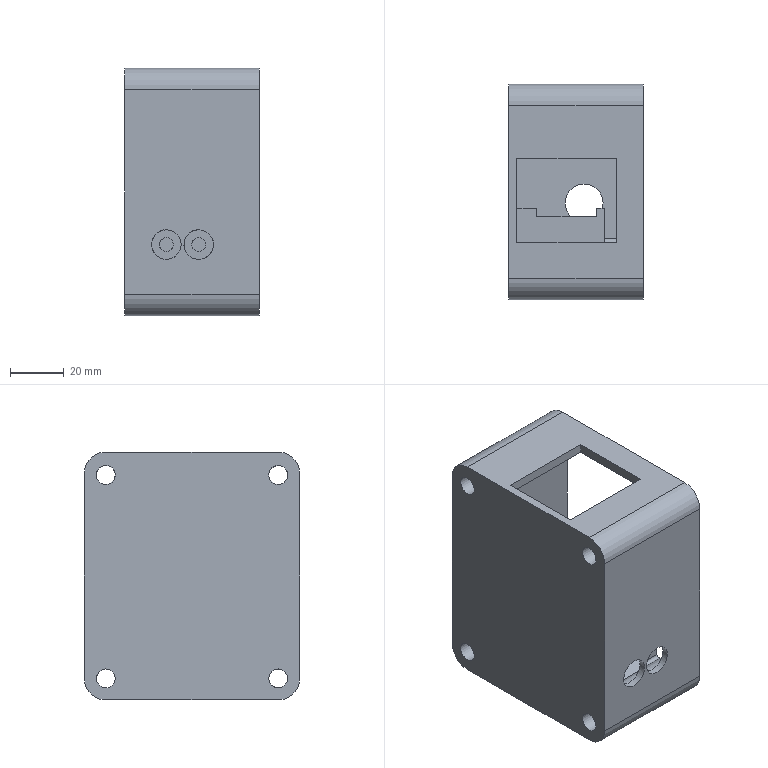NC program | NX | posted by the shop | part box 50 x 80 x 92 mm
Lines 26784 to 27158 of 30419:
(T=11 N=D6-18-D6-50-3T-rough D=6.00 R=0.00 FL=18.00 L=50.00)
(XY-STOCK=0.00)
T11 M6
T15
G0 G90 G54 X-1.75 Y-32.5 S4000 M3
G43 H11 Z30.
M8
Z-5.5
G1 Z-7.5 F800.
G3 X.25 Y-34.5 I2. J0.0
G1 X27.802
G2 X32.762 Y-22.9 I10.198 J2.5
X34.258 Y-22.5 I1.497 J-2.6
G1 X40.
Y22.5
X34.258
G2 X32.762 Y22.9 I0.0 J3.
X27.802 Y34.5 I5.238 J9.1
G1 X-27.302
G2 X-32.262 Y22.9 I-10.198 J-2.5
X-33.758 Y22.5 I-1.497 J2.6
G1 X-41.
Y-22.5
X-33.758
G2 X-32.262 Y-22.9 I0.0 J-3.
X-27.302 Y-34.5 I-5.238 J-9.1
G1 X.25
G3 X2.25 Y-32.5 I0.0 J2.
G1 Z-5.5
G0 Z30.
G0 X31.922 Y14. S4000 M3
M8
Z-5.5
G1 Z-7.5 F800.
Y18.
G3 X29.922 Y20. I-2. J0.0
G1 X-29.422
G3 X-31.422 Y18. I0.0 J-2.
G1 Y14.
Z-5.5
G0 Z30.
X31.922
Z-5.5
G1 Z-7.5
Y21.
G3 X29.922 Y23. I-2. J0.0
G1 X-29.422
G3 X-31.422 Y21. I0.0 J-2.
G1 Y14.
Z-5.5
G0 Z30.
Y-14.
Z-5.5
G1 Z-7.5
Y-18.
G3 X-29.422 Y-20. I2. J0.0
G1 X31.979
G3 X33.979 Y-18. I0.0 J2.
G1 Y-14.
Z-5.5
G0 Z30.
X-31.422
Z-5.5
G1 Z-7.5
Y-21.
G3 X-29.422 Y-23. I2. J0.0
G1 X31.979
G3 X33.979 Y-21. I0.0 J2.
G1 Y-14.
Z-5.5
G0 Z30.
G0 X-.75 Y-33.5 S4000 M3
M8
Z-15.
G1 Z-17. F800.
G3 X.25 Y-34.5 I1. J0.0
G1 X27.802
G2 X28.014 Y-28.756 I10.198 J2.5
G1 X27.257 Y-28.
X-27.792
G2 X-27.302 Y-34.5 I-9.708 J-4.
G1 X.25
G3 X1.25 Y-33.5 I0.0 J1.
G1 X-.75
G3 X.25 Y-34.5 I1. J0.0
G1 X27.802
G2 X28.014 Y-28.756 I10.198 J2.5
G1 X27.257 Y-28.
X-27.792
G2 X-27.302 Y-34.5 I-9.708 J-4.
G1 X.25
G3 X1.25 Y-33.5 I0.0 J1.
G1 Z-15.
G0 Z30.
Y33.5
Z-15.
G1 Z-17.
G3 X.25 Y34.5 I-1. J0.0
G1 X-27.302
G2 X-27.792 Y28. I-10.198 J-2.5
G1 X28.292
G2 X27.802 Y34.5 I9.708 J4.
G1 X.25
G3 X-.75 Y33.5 I0.0 J-1.
G1 X1.25
G3 X.25 Y34.5 I-1. J0.0
G1 X-27.302
G2 X-27.792 Y28. I-10.198 J-2.5
G1 X28.292
G2 X27.802 Y34.5 I9.708 J4.
G1 X.25
G3 X-.75 Y33.5 I0.0 J-1.
G1 Z-15.
G0 Z30.
G0 X3. Y-.402 S4000 M3
M8
Z-11.5
G1 Z-14.5 F800.
Y-6.
G3 X4.5 Y-7.5 I1.5 J0.0
G1 X30.5
Y-11.333
X4.5
Y-15.167
X30.5
X31.743 Y-19.
X4.696
Z-11.5
G0 Z30.
M9
M5
G91 G28 Z0.0
M1
N9
(T=15 N=D6-18-D6-50-3T-rough D=6.00 R=0.00 FL=18.00 L=50.00)
(XY-STOCK=0.00)
T15 M6
T8
G0 G90 G54 X-37.5 Y2. S4000 M3
G43 H15 Z30.
M8
Z-45.
G1 Z-47. F800.
G3 X-39.5 Y0.0 I0.0 J-2.
G1 Y-16.084
G2 X-35.304 Y-19. I-1. J-5.916
G1 X-5.696
G2 X4.104 Y-18.153 I5.196 J-3.
G1 X4.5 Y-17.757
Y-6.
G2 X7.5 Y-3. I3. J0.0
G1 X27.5
G2 X30.5 Y-6. I0.0 J-3.
G1 Y-17.757
X31.743 Y-19.
X34.304
G2 X38.5 Y-16.084 I5.196 J-3.
G1 Y16.084
G2 X34.304 Y19. I1. J5.916
G1 X4.696
G2 X-5.696 I-5.196 J3.
G1 X-35.304
G2 X-39.5 Y16.084 I-5.196 J3.
G1 Y0.0
G3 X-37.5 Y-2. I2. J0.0
G1 Y2.
G3 X-39.5 Y0.0 I0.0 J-2.
G1 Y-16.084
G2 X-35.304 Y-19. I-1. J-5.916
G1 X-5.696
G2 X4.104 Y-18.153 I5.196 J-3.
G1 X4.5 Y-17.757
Y-6.
G2 X7.5 Y-3. I3. J0.0
G1 X27.5
G2 X30.5 Y-6. I0.0 J-3.
G1 Y-17.757
X31.743 Y-19.
X34.304
G2 X38.5 Y-16.084 I5.196 J-3.
G1 Y16.084
G2 X34.304 Y19. I1. J5.916
G1 X4.696
G2 X-5.696 I-5.196 J3.
G1 X-35.304
G2 X-39.5 Y16.084 I-5.196 J3.
G1 Y0.0
G3 X-37.5 Y-2. I2. J0.0
G1 Y2.
G3 X-39.5 Y0.0 I0.0 J-2.
G1 Y-16.084
G2 X-35.304 Y-19. I-1. J-5.916
G1 X-5.696
G2 X4.104 Y-18.153 I5.196 J-3.
G1 X4.5 Y-17.757
Y-6.
G2 X7.5 Y-3. I3. J0.0
G1 X27.5
G2 X30.5 Y-6. I0.0 J-3.
G1 Y-17.757
X31.743 Y-19.
X34.304
G2 X38.5 Y-16.084 I5.196 J-3.
G1 Y16.084
G2 X34.304 Y19. I1. J5.916
G1 X4.696
G2 X-5.696 I-5.196 J3.
G1 X-35.304
G2 X-39.5 Y16.084 I-5.196 J3.
G1 Y0.0
G3 X-37.5 Y-2. I2. J0.0
G1 Y2.
G3 X-39.5 Y0.0 I0.0 J-2.
G1 Y-16.084
G2 X-35.304 Y-19. I-1. J-5.916
G1 X-5.696
G2 X4.104 Y-18.153 I5.196 J-3.
G1 X4.5 Y-17.757
Y-6.
G2 X7.5 Y-3. I3. J0.0
G1 X27.5
G2 X30.5 Y-6. I0.0 J-3.
G1 Y-17.757
X31.743 Y-19.
X34.304
G2 X38.5 Y-16.084 I5.196 J-3.
G1 Y16.084
G2 X34.304 Y19. I1. J5.916
G1 X4.696
G2 X-5.696 I-5.196 J3.
G1 X-35.304
G2 X-39.5 Y16.084 I-5.196 J3.
G1 Y0.0
G3 X-37.5 Y-2. I2. J0.0
G1 Y2.
G3 X-39.5 Y0.0 I0.0 J-2.
G1 Y-16.084
G2 X-35.304 Y-19. I-1. J-5.916
G1 X-5.696
G2 X4.104 Y-18.153 I5.196 J-3.
G1 X4.5 Y-17.757
Y-6.
G2 X7.5 Y-3. I3. J0.0
G1 X27.5
G2 X30.5 Y-6. I0.0 J-3.
G1 Y-17.757
X31.743 Y-19.
X34.304
G2 X38.5 Y-16.084 I5.196 J-3.
G1 Y16.084
G2 X34.304 Y19. I1. J5.916
G1 X4.696
G2 X-5.696 I-5.196 J3.
G1 X-35.304
G2 X-39.5 Y16.084 I-5.196 J3.
G1 Y0.0
G3 X-37.5 Y-2. I2. J0.0
G1 Z-45.
G0 Z30.
G0 X-.75 Y-33.5 S4000 M3
M8
Z-45.
G1 Z-47. F800.
G3 X.25 Y-34.5 I1. J0.0
G1 X27.802
G2 X28.014 Y-28.756 I10.198 J2.5
G1 X27.257 Y-28.
X-27.792
G2 X-27.302 Y-34.5 I-9.708 J-4.
G1 X.25
G3 X1.25 Y-33.5 I0.0 J1.
G1 X-.75
G3 X.25 Y-34.5 I1. J0.0
G1 X27.802
G2 X28.014 Y-28.756 I10.198 J2.5
G1 X27.257 Y-28.
X-27.792
G2 X-27.302 Y-34.5 I-9.708 J-4.
G1 X.25
G3 X1.25 Y-33.5 I0.0 J1.
G1 X-.75
G3 X.25 Y-34.5 I1. J0.0
G1 X27.802
G2 X28.014 Y-28.756 I10.198 J2.5
G1 X27.257 Y-28.
X-27.792
G2 X-27.302 Y-34.5 I-9.708 J-4.
G1 X.25
G3 X1.25 Y-33.5 I0.0 J1.
G1 X-.75
G3 X.25 Y-34.5 I1. J0.0
G1 X27.802
G2 X28.014 Y-28.756 I10.198 J2.5
G1 X27.257 Y-28.
X-27.792
G2 X-27.302 Y-34.5 I-9.708 J-4.
G1 X.25
G3 X1.25 Y-33.5 I0.0 J1.
G1 X-.75
G3 X.25 Y-34.5 I1. J0.0
G1 X27.802
G2 X28.014 Y-28.756 I10.198 J2.5
G1 X27.257 Y-28.
X-27.792
G2 X-27.302 Y-34.5 I-9.708 J-4.
G1 X.25
G3 X1.25 Y-33.5 I0.0 J1.
G1 X-.75
G3 X.25 Y-34.5 I1. J0.0
G1 X27.802
G2 X28.014 Y-28.756 I10.198 J2.5
G1 X27.257 Y-28.
X-27.792
G2 X-27.302 Y-34.5 I-9.708 J-4.
G1 X.25
G3 X1.25 Y-33.5 I0.0 J1.
G1 Z-45.
G0 Z30.
Y33.5
Z-45.
G1 Z-47.
G3 X.25 Y34.5 I-1. J0.0
G1 X-27.302
G2 X-27.792 Y28. I-10.198 J-2.5
G1 X28.292
G2 X27.802 Y34.5 I9.708 J4.
G1 X.25
G3 X-.75 Y33.5 I0.0 J-1.
G1 X1.25
G3 X.25 Y34.5 I-1. J0.0
G1 X-27.302
G2 X-27.792 Y28. I-10.198 J-2.5
G1 X28.292
G2 X27.802 Y34.5 I9.708 J4.
G1 X.25
G3 X-.75 Y33.5 I0.0 J-1.
G1 X1.25
G3 X.25 Y34.5 I-1. J0.0
G1 X-27.302
G2 X-27.792 Y28. I-10.198 J-2.5
G1 X28.292
G2 X27.802 Y34.5 I9.708 J4.
G1 X.25
G3 X-.75 Y33.5 I0.0 J-1.
G1 X1.25
G3 X.25 Y34.5 I-1. J0.0
G1 X-27.302
G2 X-27.792 Y28. I-10.198 J-2.5
G1 X28.292
G2 X27.802 Y34.5 I9.708 J4.
G1 X.25
G3 X-.75 Y33.5 I0.0 J-1.
G1 X1.25
G3 X.25 Y34.5 I-1. J0.0
G1 X-27.302
G2 X-27.792 Y28. I-10.198 J-2.5
G1 X28.292
G2 X27.802 Y34.5 I9.708 J4.
G1 X.25
G3 X-.75 Y33.5 I0.0 J-1.
G1 X1.25
G3 X.25 Y34.5 I-1. J0.0
G1 X-27.302
G2 X-27.792 Y28. I-10.198 J-2.5
G1 X28.292
G2 X27.802 Y34.5 I9.708 J4.
G1 X.25
G3 X-.75 Y33.5 I0.0 J-1.
G1 Z-45.
G0 Z30.
M9
M5
G91 G28 Z0.0
M1
N10